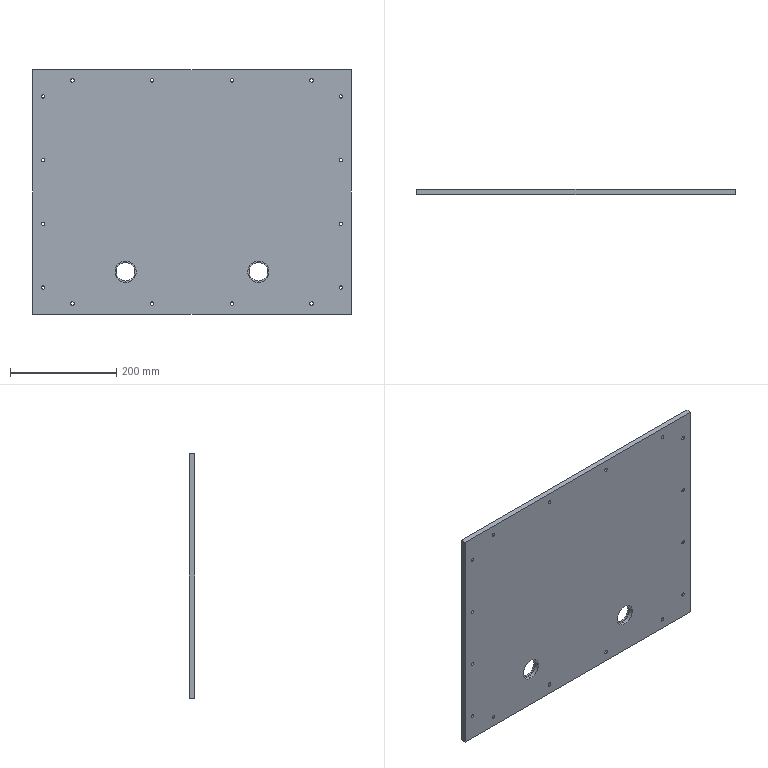Part | STEP file | Bracket二后立Plate | 1 solid | 80 faces | box 600 x 10 x 460 mm | volume 2728752 mm3 | cylinder 40 | cone 32 | plane 8 | commonest cylinder face diameters 6.6 x32 35 x4 40 x4